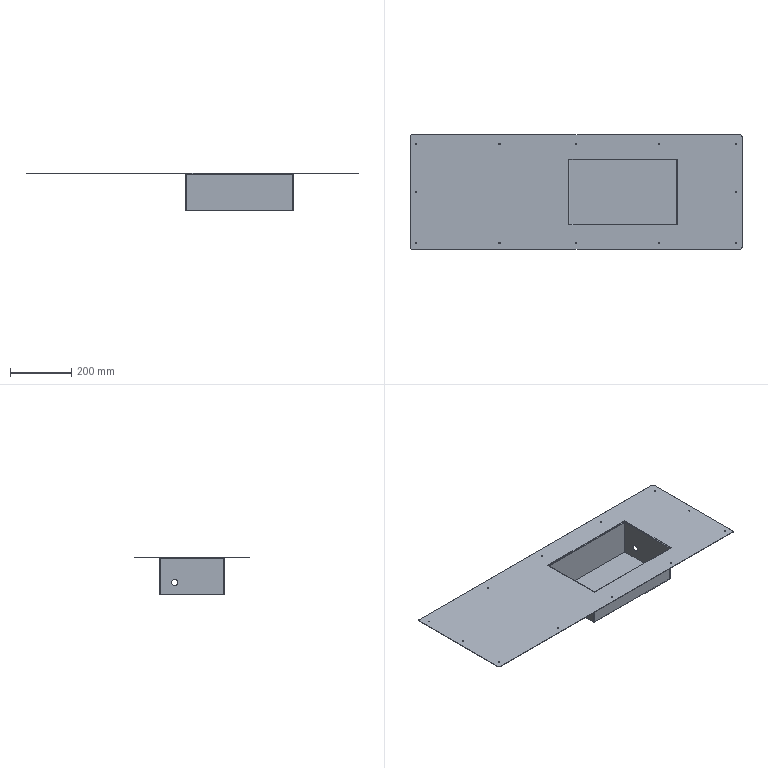Part | SolidWorks | features ICE 4, Fillet 2, EdgeFlange 1, FlatPattern 1, SMBaseFlange 1, SheetMetal 1 | 1 solid | 76 faces | box 1087 x 374 x 123 mm | volume 809461 mm3 | cylinder 44 | plane 24 | spline 8 | commonest cylinder face diameters 5 x28 3 x4 6 x4 10 x4 20 x4